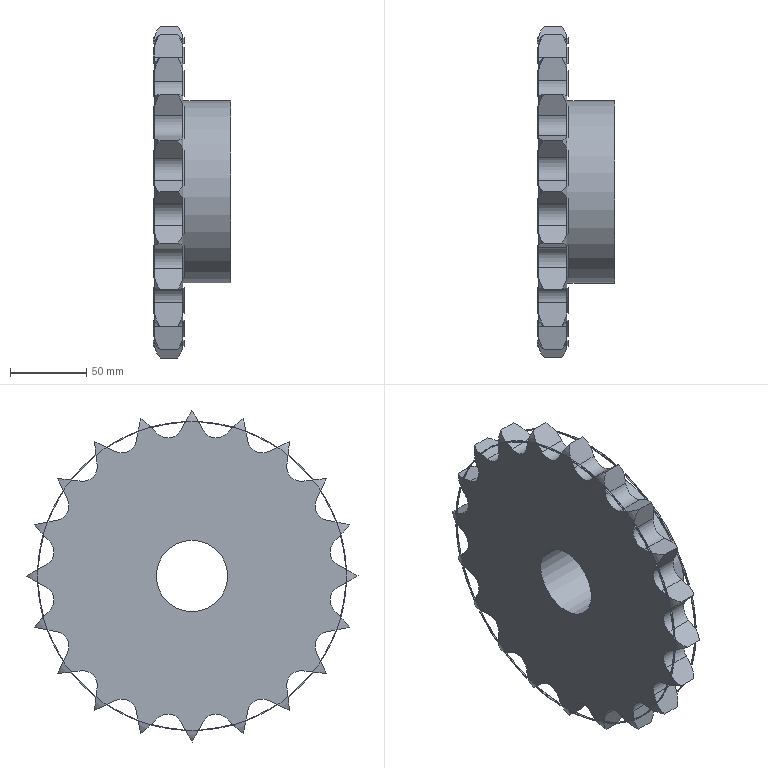Part | STEP file | single_steel_sprocket_step_31_75mm_pgs31720mBK | 41 solids | 345 faces | box 51 x 218.1 x 218.1 mm | volume 824761 mm3 | plane 203 | cylinder 102 | torus 40 | commonest cylinder face diameters 202.11 x40 202.98 x40 19.05 x20 47 x1 120 x1